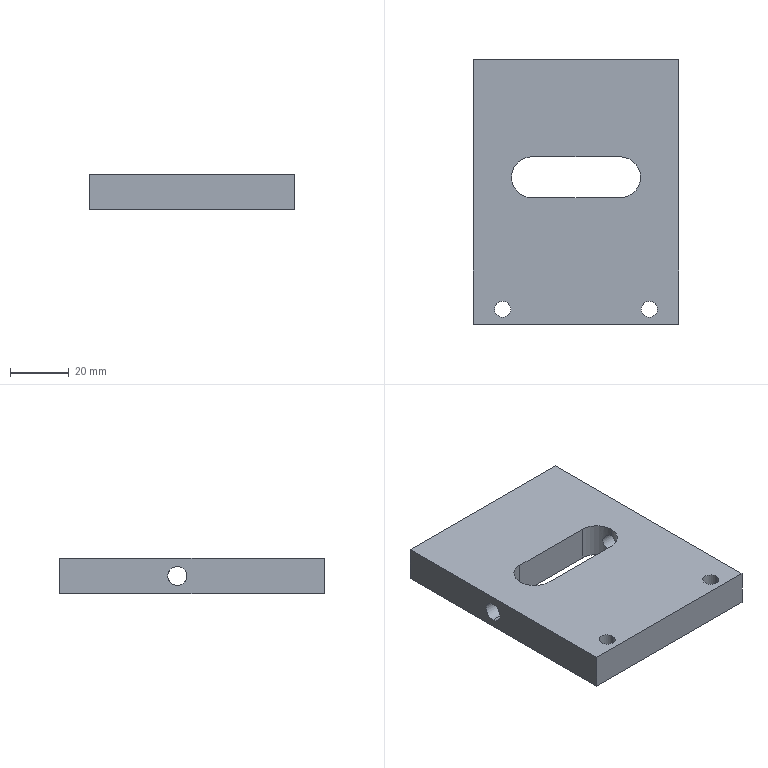Part | SolidWorks | features ICE 2, Cut 1, Extrusion 1, HoleWzd 1 | 1 solid | 27 faces | box 70 x 90 x 12 mm | volume 66580 mm3 | cylinder 15 | plane 8 | cone 4 | commonest cylinder face diameters 5 x4 5.5 x4 6.5 x4 14 x3
STEP:
#1=CARTESIAN_POINT('',(57.25,-85.,0.));
#2=VERTEX_POINT('',#1);
#3=CARTESIAN_POINT('',(62.75,-85.,0.));
#4=VERTEX_POINT('',#3);
#5=CARTESIAN_POINT('',(60.,-85.,0.));
#6=DIRECTION('',(0.,0.,1.));
#7=DIRECTION('',(1.,0.,0.));
#8=AXIS2_PLACEMENT_3D('',#5,#6,#7);
#9=CIRCLE('',#8,2.75);
#10=EDGE_CURVE('',#2,#4,#9,.T.);
#11=ORIENTED_EDGE('',*,*,#10,.F.);
#12=CARTESIAN_POINT('',(57.25,-85.,12.));
#13=VERTEX_POINT('',#12);
#14=CARTESIAN_POINT('',(57.25,-85.,0.));
#15=DIRECTION('',(0.,0.,1.));
#16=VECTOR('',#15,1000.);
#17=LINE('',#14,#16);
#18=EDGE_CURVE('',#2,#13,#17,.T.);
#19=ORIENTED_EDGE('',*,*,#18,.T.);
#20=CARTESIAN_POINT('',(62.75,-85.,12.));
#21=VERTEX_POINT('',#20);
#22=CARTESIAN_POINT('',(60.,-85.,12.));
#23=DIRECTION('',(0.,0.,1.));
#24=DIRECTION('',(1.,0.,0.));
#25=AXIS2_PLACEMENT_3D('',#22,#23,#24);
#26=CIRCLE('',#25,2.75);
#27=EDGE_CURVE('',#13,#21,#26,.T.);
#28=ORIENTED_EDGE('',*,*,#27,.T.);
#29=CARTESIAN_POINT('',(62.75,-85.,0.));
#30=DIRECTION('',(0.,0.,1.));
#31=VECTOR('',#30,1000.);
#32=LINE('',#29,#31);
#33=EDGE_CURVE('',#4,#21,#32,.T.);
#34=ORIENTED_EDGE('',*,*,#33,.F.);
#35=EDGE_LOOP('',(#11,#19,#28,#34));
#36=FACE_OUTER_BOUND('',#35,.T.);
#37=CARTESIAN_POINT('',(60.,-85.,0.));
#38=DIRECTION('',(0.,0.,1.));
#39=DIRECTION('',(1.,0.,0.));
#40=AXIS2_PLACEMENT_3D('',#37,#38,#39);
#41=CYLINDRICAL_SURFACE('',#40,2.75);
#42=ADVANCED_FACE('',(#36),#41,.F.);
#43=CARTESIAN_POINT('',(7.25,-85.,0.));
#44=VERTEX_POINT('',#43);
#45=CARTESIAN_POINT('',(12.75,-85.,0.));
#46=VERTEX_POINT('',#45);
#47=CARTESIAN_POINT('',(10.,-85.,0.));
#48=DIRECTION('',(0.,0.,1.));
#49=DIRECTION('',(1.,0.,0.));
#50=AXIS2_PLACEMENT_3D('',#47,#48,#49);
#51=CIRCLE('',#50,2.75);
#52=EDGE_CURVE('',#44,#46,#51,.T.);
#53=ORIENTED_EDGE('',*,*,#52,.F.);
#54=CARTESIAN_POINT('',(7.25,-85.,12.));
#55=VERTEX_POINT('',#54);
#56=CARTESIAN_POINT('',(7.25,-85.,0.));
#57=DIRECTION('',(0.,0.,1.));
#58=VECTOR('',#57,1000.);
#59=LINE('',#56,#58);
#60=EDGE_CURVE('',#44,#55,#59,.T.);
#61=ORIENTED_EDGE('',*,*,#60,.T.);
#62=CARTESIAN_POINT('',(12.75,-85.,12.));
#63=VERTEX_POINT('',#62);
#64=CARTESIAN_POINT('',(10.,-85.,12.));
#65=DIRECTION('',(0.,0.,1.));
#66=DIRECTION('',(1.,0.,0.));
#67=AXIS2_PLACEMENT_3D('',#64,#65,#66);
#68=CIRCLE('',#67,2.75);
#69=EDGE_CURVE('',#55,#63,#68,.T.);
#70=ORIENTED_EDGE('',*,*,#69,.T.);
#71=CARTESIAN_POINT('',(12.75,-85.,0.));
#72=DIRECTION('',(0.,0.,1.));
#73=VECTOR('',#72,1000.);
#74=LINE('',#71,#73);
#75=EDGE_CURVE('',#46,#63,#74,.T.);
#76=ORIENTED_EDGE('',*,*,#75,.F.);
#77=EDGE_LOOP('',(#53,#61,#70,#76));
#78=FACE_OUTER_BOUND('',#77,.T.);
#79=CARTESIAN_POINT('',(10.,-85.,0.));
#80=DIRECTION('',(0.,0.,1.));
#81=DIRECTION('',(1.,0.,0.));
#82=AXIS2_PLACEMENT_3D('',#79,#80,#81);
#83=CYLINDRICAL_SURFACE('',#82,2.75);
#84=ADVANCED_FACE('',(#78),#83,.F.);
#85=CARTESIAN_POINT('',(62.5,-17.,3.5));
#86=VERTEX_POINT('',#85);
#87=CARTESIAN_POINT('',(62.5,-17.,8.5));
#88=VERTEX_POINT('',#87);
#89=CARTESIAN_POINT('',(62.5,-17.,6.));
#90=DIRECTION('',(0.,1.,0.));
#91=DIRECTION('',(0.,0.,1.));
#92=AXIS2_PLACEMENT_3D('',#89,#90,#91);
#93=CIRCLE('',#92,2.5);
#94=EDGE_CURVE('',#86,#88,#93,.T.);
#95=ORIENTED_EDGE('',*,*,#94,.F.);
#96=CARTESIAN_POINT('',(62.5,0.,3.5));
#97=VERTEX_POINT('',#96);
#98=CARTESIAN_POINT('',(62.5,0.,3.5));
#99=DIRECTION('',(0.,1.,0.));
#100=VECTOR('',#99,1000.);
#101=LINE('',#98,#100);
#102=EDGE_CURVE('',#86,#97,#101,.T.);
#103=ORIENTED_EDGE('',*,*,#102,.T.);
#104=CARTESIAN_POINT('',(62.5,0.,8.5));
#105=VERTEX_POINT('',#104);
#106=CARTESIAN_POINT('',(62.5,0.,6.));
#107=DIRECTION('',(0.,1.,0.));
#108=DIRECTION('',(0.,0.,1.));
#109=AXIS2_PLACEMENT_3D('',#106,#107,#108);
#110=CIRCLE('',#109,2.5);
#111=EDGE_CURVE('',#97,#105,#110,.T.);
#112=ORIENTED_EDGE('',*,*,#111,.T.);
#113=CARTESIAN_POINT('',(62.5,0.,8.5));
#114=DIRECTION('',(0.,1.,0.));
#115=VECTOR('',#114,1000.);
#116=LINE('',#113,#115);
#117=EDGE_CURVE('',#88,#105,#116,.T.);
#118=ORIENTED_EDGE('',*,*,#117,.F.);
#119=EDGE_LOOP('',(#95,#103,#112,#118));
#120=FACE_OUTER_BOUND('',#119,.T.);
#121=CARTESIAN_POINT('',(62.5,0.,6.));
#122=DIRECTION('',(0.,1.,0.));
#123=DIRECTION('',(0.,0.,1.));
#124=AXIS2_PLACEMENT_3D('',#121,#122,#123);
#125=CYLINDRICAL_SURFACE('',#124,2.5);
#126=ADVANCED_FACE('',(#120),#125,.F.);
#127=CARTESIAN_POINT('',(62.5,-18.502,6.));
#128=VERTEX_POINT('',#127);
#129=CARTESIAN_POINT('',(62.5,-17.,8.5));
#130=DIRECTION('',(0.,0.515,0.8572));
#131=VECTOR('',#130,1000.);
#132=LINE('',#129,#131);
#133=EDGE_CURVE('',#128,#88,#132,.T.);
#134=ORIENTED_EDGE('',*,*,#133,.F.);
#135=CARTESIAN_POINT('',(62.5,-17.,3.5));
#136=DIRECTION('',(0.,0.515,-0.8572));
#137=VECTOR('',#136,1000.);
#138=LINE('',#135,#137);
#139=EDGE_CURVE('',#128,#86,#138,.T.);
#140=ORIENTED_EDGE('',*,*,#139,.T.);
#141=ORIENTED_EDGE('',*,*,#94,.T.);
#142=EDGE_LOOP('',(#134,#140,#141));
#143=FACE_OUTER_BOUND('',#142,.T.);
#144=CARTESIAN_POINT('',(62.5,-17.,6.));
#145=DIRECTION('',(0.,1.,0.));
#146=DIRECTION('',(0.,0.,1.));
#147=AXIS2_PLACEMENT_3D('',#144,#145,#146);
#148=CONICAL_SURFACE('',#147,2.5,1.03);
#149=ADVANCED_FACE('',(#143),#148,.F.);
#150=CARTESIAN_POINT('',(7.5,-17.,3.5));
#151=VERTEX_POINT('',#150);
#152=CARTESIAN_POINT('',(7.5,-17.,8.5));
#153=VERTEX_POINT('',#152);
#154=CARTESIAN_POINT('',(7.5,-17.,6.));
#155=DIRECTION('',(0.,1.,0.));
#156=DIRECTION('',(0.,0.,1.));
#157=AXIS2_PLACEMENT_3D('',#154,#155,#156);
#158=CIRCLE('',#157,2.5);
#159=EDGE_CURVE('',#151,#153,#158,.T.);
#160=ORIENTED_EDGE('',*,*,#159,.F.);
#161=CARTESIAN_POINT('',(7.5,0.,3.5));
#162=VERTEX_POINT('',#161);
#163=CARTESIAN_POINT('',(7.5,0.,3.5));
#164=DIRECTION('',(0.,1.,0.));
#165=VECTOR('',#164,1000.);
#166=LINE('',#163,#165);
#167=EDGE_CURVE('',#151,#162,#166,.T.);
#168=ORIENTED_EDGE('',*,*,#167,.T.);
#169=CARTESIAN_POINT('',(7.5,0.,8.5));
#170=VERTEX_POINT('',#169);
#171=CARTESIAN_POINT('',(7.5,0.,6.));
#172=DIRECTION('',(0.,1.,0.));
#173=DIRECTION('',(0.,0.,1.));
#174=AXIS2_PLACEMENT_3D('',#171,#172,#173);
#175=CIRCLE('',#174,2.5);
#176=EDGE_CURVE('',#162,#170,#175,.T.);
#177=ORIENTED_EDGE('',*,*,#176,.T.);
#178=CARTESIAN_POINT('',(7.5,0.,8.5));
#179=DIRECTION('',(0.,1.,0.));
#180=VECTOR('',#179,1000.);
#181=LINE('',#178,#180);
#182=EDGE_CURVE('',#153,#170,#181,.T.);
#183=ORIENTED_EDGE('',*,*,#182,.F.);
#184=EDGE_LOOP('',(#160,#168,#177,#183));
#185=FACE_OUTER_BOUND('',#184,.T.);
#186=CARTESIAN_POINT('',(7.5,0.,6.));
#187=DIRECTION('',(0.,1.,0.));
#188=DIRECTION('',(0.,0.,1.));
#189=AXIS2_PLACEMENT_3D('',#186,#187,#188);
#190=CYLINDRICAL_SURFACE('',#189,2.5);
#191=ADVANCED_FACE('',(#185),#190,.F.);
#192=CARTESIAN_POINT('',(7.5,-18.502,6.));
#193=VERTEX_POINT('',#192);
#194=CARTESIAN_POINT('',(7.5,-17.,8.5));
#195=DIRECTION('',(0.,0.515,0.8572));
#196=VECTOR('',#195,1000.);
#197=LINE('',#194,#196);
#198=EDGE_CURVE('',#193,#153,#197,.T.);
#199=ORIENTED_EDGE('',*,*,#198,.F.);
#200=CARTESIAN_POINT('',(7.5,-17.,3.5));
#201=DIRECTION('',(0.,0.515,-0.8572));
#202=VECTOR('',#201,1000.);
#203=LINE('',#200,#202);
#204=EDGE_CURVE('',#193,#151,#203,.T.);
#205=ORIENTED_EDGE('',*,*,#204,.T.);
#206=ORIENTED_EDGE('',*,*,#159,.T.);
#207=EDGE_LOOP('',(#199,#205,#206));
#208=FACE_OUTER_BOUND('',#207,.T.);
#209=CARTESIAN_POINT('',(7.5,-17.,6.));
#210=DIRECTION('',(0.,1.,0.));
#211=DIRECTION('',(0.,0.,1.));
#212=AXIS2_PLACEMENT_3D('',#209,#210,#211);
#213=CONICAL_SURFACE('',#212,2.5,1.03);
#214=ADVANCED_FACE('',(#208),#213,.F.);
#215=CARTESIAN_POINT('',(0.,-40.,9.25));
#216=VERTEX_POINT('',#215);
#217=CARTESIAN_POINT('',(0.,-40.,2.75));
#218=VERTEX_POINT('',#217);
#219=CARTESIAN_POINT('',(0.,-40.,6.));
#220=DIRECTION('',(1.,0.,0.));
#221=DIRECTION('',(0.,0.,-1.));
#222=AXIS2_PLACEMENT_3D('',#219,#220,#221);
#223=CIRCLE('',#222,3.25);
#224=EDGE_CURVE('',#216,#218,#223,.T.);
#225=ORIENTED_EDGE('',*,*,#224,.F.);
#226=CARTESIAN_POINT('',(13.,-40.,9.25));
#227=VERTEX_POINT('',#226);
#228=CARTESIAN_POINT('',(0.,-40.,9.25));
#229=DIRECTION('',(1.,0.,0.));
#230=VECTOR('',#229,1000.);
#231=LINE('',#228,#230);
#232=EDGE_CURVE('',#216,#227,#231,.T.);
#233=ORIENTED_EDGE('',*,*,#232,.T.);
#234=CARTESIAN_POINT('',(13.,-40.,2.75));
#235=VERTEX_POINT('',#234);
#236=CARTESIAN_POINT('',(13.,-40.,2.75));
#237=CARTESIAN_POINT('',(13.,-40.218,2.75));
#238=CARTESIAN_POINT('',(13.01,-40.432,2.772));
#239=CARTESIAN_POINT('',(13.049,-40.852,2.856));
#240=CARTESIAN_POINT('',(13.078,-41.06,2.92));
#241=CARTESIAN_POINT('',(13.149,-41.453,3.085));
#242=CARTESIAN_POINT('',(13.192,-41.638,3.185));
#243=CARTESIAN_POINT('',(13.286,-41.989,3.421));
#244=CARTESIAN_POINT('',(13.337,-42.153,3.556));
#245=CARTESIAN_POINT('',(13.44,-42.448,3.852));
#246=CARTESIAN_POINT('',(13.492,-42.582,4.015));
#247=CARTESIAN_POINT('',(13.591,-42.817,4.366));
#248=CARTESIAN_POINT('',(13.636,-42.917,4.551));
#249=CARTESIAN_POINT('',(13.713,-43.08,4.94));
#250=CARTESIAN_POINT('',(13.745,-43.144,5.148));
#251=CARTESIAN_POINT('',(13.789,-43.228,5.569));
#252=CARTESIAN_POINT('',(13.8,-43.25,5.782));
#253=CARTESIAN_POINT('',(13.8,-43.25,6.213));
#254=CARTESIAN_POINT('',(13.789,-43.228,6.432));
#255=CARTESIAN_POINT('',(13.745,-43.144,6.852));
#256=CARTESIAN_POINT('',(13.714,-43.081,7.057));
#257=CARTESIAN_POINT('',(13.635,-42.916,7.452));
#258=CARTESIAN_POINT('',(13.59,-42.816,7.637));
#259=CARTESIAN_POINT('',(13.492,-42.581,7.986));
#260=CARTESIAN_POINT('',(13.439,-42.446,8.151));
#261=CARTESIAN_POINT('',(13.336,-42.15,8.446));
#262=CARTESIAN_POINT('',(13.286,-41.988,8.579));
#263=CARTESIAN_POINT('',(13.192,-41.637,8.816));
#264=CARTESIAN_POINT('',(13.149,-41.449,8.917));
#265=CARTESIAN_POINT('',(13.078,-41.059,9.08));
#266=CARTESIAN_POINT('',(13.049,-40.854,9.143));
#267=CARTESIAN_POINT('',(13.01,-40.429,9.229));
#268=CARTESIAN_POINT('',(13.,-40.215,9.25));
#269=CARTESIAN_POINT('',(13.,-40.,9.25));
#270=B_SPLINE_CURVE_WITH_KNOTS('',3,(#236,#237,#238,#239,#240,#241,#242,#243,#244,#245,#246,#247,#248,#249,#250,#251,#252,#253,#254,#255,#256,#257,#258,#259,#260,#261,#262,#263,#264,#265,#266,#267,#268,#269),.UNSPECIFIED.,.F.,.F.,(4,2,2,2,2,2,2,2,2,2,2,2,2,2,2,2,4),(0.,0.0006445,0.001289,0.001933,0.002578,0.003222,0.003867,0.004511,0.005156,0.0058,0.006445,0.007089,0.007733,0.008378,0.009022,0.009667,0.01031),.UNSPECIFIED.);
#271=EDGE_CURVE('',#235,#227,#270,.T.);
#272=ORIENTED_EDGE('',*,*,#271,.F.);
#273=CARTESIAN_POINT('',(0.,-40.,2.75));
#274=DIRECTION('',(1.,0.,0.));
#275=VECTOR('',#274,1000.);
#276=LINE('',#273,#275);
#277=EDGE_CURVE('',#218,#235,#276,.T.);
#278=ORIENTED_EDGE('',*,*,#277,.F.);
#279=EDGE_LOOP('',(#225,#233,#272,#278));
#280=FACE_OUTER_BOUND('',#279,.T.);
#281=CARTESIAN_POINT('',(0.,-40.,6.));
#282=DIRECTION('',(1.,0.,0.));
#283=DIRECTION('',(0.,0.,-1.));
#284=AXIS2_PLACEMENT_3D('',#281,#282,#283);
#285=CYLINDRICAL_SURFACE('',#284,3.25);
#286=ADVANCED_FACE('',(#280),#285,.F.);
#287=CARTESIAN_POINT('',(57.,-40.,9.25));
#288=VERTEX_POINT('',#287);
#289=CARTESIAN_POINT('',(57.,-40.,2.75));
#290=VERTEX_POINT('',#289);
#291=CARTESIAN_POINT('',(57.,-40.,9.25));
#292=CARTESIAN_POINT('',(57.,-40.215,9.25));
#293=CARTESIAN_POINT('',(56.99,-40.433,9.228));
#294=CARTESIAN_POINT('',(56.951,-40.854,9.143));
#295=CARTESIAN_POINT('',(56.922,-41.058,9.08));
#296=CARTESIAN_POINT('',(56.851,-41.453,8.915));
#297=CARTESIAN_POINT('',(56.808,-41.64,8.814));
#298=CARTESIAN_POINT('',(56.714,-41.989,8.579));
#299=CARTESIAN_POINT('',(56.663,-42.153,8.444));
#300=CARTESIAN_POINT('',(56.559,-42.449,8.147));
#301=CARTESIAN_POINT('',(56.508,-42.581,7.986));
#302=CARTESIAN_POINT('',(56.41,-42.815,7.637));
#303=CARTESIAN_POINT('',(56.364,-42.917,7.448));
#304=CARTESIAN_POINT('',(56.287,-43.08,7.058));
#305=CARTESIAN_POINT('',(56.255,-43.143,6.856));
#306=CARTESIAN_POINT('',(56.211,-43.228,6.434));
#307=CARTESIAN_POINT('',(56.2,-43.25,6.217));
#308=CARTESIAN_POINT('',(56.2,-43.25,5.788));
#309=CARTESIAN_POINT('',(56.211,-43.229,5.572));
#310=CARTESIAN_POINT('',(56.255,-43.144,5.148));
#311=CARTESIAN_POINT('',(56.286,-43.081,4.944));
#312=CARTESIAN_POINT('',(56.364,-42.918,4.552));
#313=CARTESIAN_POINT('',(56.41,-42.816,4.364));
#314=CARTESIAN_POINT('',(56.508,-42.582,4.015));
#315=CARTESIAN_POINT('',(56.56,-42.449,3.853));
#316=CARTESIAN_POINT('',(56.663,-42.15,3.554));
#317=CARTESIAN_POINT('',(56.714,-41.989,3.421));
#318=CARTESIAN_POINT('',(56.807,-41.641,3.187));
#319=CARTESIAN_POINT('',(56.851,-41.452,3.085));
#320=CARTESIAN_POINT('',(56.922,-41.059,2.92));
#321=CARTESIAN_POINT('',(56.951,-40.856,2.857));
#322=CARTESIAN_POINT('',(56.99,-40.436,2.772));
#323=CARTESIAN_POINT('',(57.,-40.218,2.75));
#324=CARTESIAN_POINT('',(57.,-40.,2.75));
#325=B_SPLINE_CURVE_WITH_KNOTS('',3,(#291,#292,#293,#294,#295,#296,#297,#298,#299,#300,#301,#302,#303,#304,#305,#306,#307,#308,#309,#310,#311,#312,#313,#314,#315,#316,#317,#318,#319,#320,#321,#322,#323,#324),.UNSPECIFIED.,.F.,.F.,(4,2,2,2,2,2,2,2,2,2,2,2,2,2,2,2,4),(0.01031,0.01095,0.0116,0.01224,0.01289,0.01353,0.01417,0.01482,0.01546,0.0161,0.01675,0.01739,0.01803,0.01868,0.01932,0.01997,0.02061),.UNSPECIFIED.);
#326=EDGE_CURVE('',#288,#290,#325,.T.);
#327=ORIENTED_EDGE('',*,*,#326,.F.);
#328=CARTESIAN_POINT('',(70.,-40.,9.25));
#329=VERTEX_POINT('',#328);
#330=CARTESIAN_POINT('',(0.,-40.,9.25));
#331=DIRECTION('',(1.,0.,0.));
#332=VECTOR('',#331,1000.);
#333=LINE('',#330,#332);
#334=EDGE_CURVE('',#288,#329,#333,.T.);
#335=ORIENTED_EDGE('',*,*,#334,.T.);
#336=CARTESIAN_POINT('',(70.,-40.,2.75));
#337=VERTEX_POINT('',#336);
#338=CARTESIAN_POINT('',(70.,-40.,6.));
#339=DIRECTION('',(1.,0.,0.));
#340=DIRECTION('',(0.,0.,-1.));
#341=AXIS2_PLACEMENT_3D('',#338,#339,#340);
#342=CIRCLE('',#341,3.25);
#343=EDGE_CURVE('',#329,#337,#342,.T.);
#344=ORIENTED_EDGE('',*,*,#343,.T.);
#345=CARTESIAN_POINT('',(0.,-40.,2.75));
#346=DIRECTION('',(1.,0.,0.));
#347=VECTOR('',#346,1000.);
#348=LINE('',#345,#347);
#349=EDGE_CURVE('',#290,#337,#348,.T.);
#350=ORIENTED_EDGE('',*,*,#349,.F.);
#351=EDGE_LOOP('',(#327,#335,#344,#350));
#352=FACE_OUTER_BOUND('',#351,.T.);
#353=CARTESIAN_POINT('',(0.,-40.,6.));
#354=DIRECTION('',(1.,0.,0.));
#355=DIRECTION('',(0.,0.,-1.));
#356=AXIS2_PLACEMENT_3D('',#353,#354,#355);
#357=CYLINDRICAL_SURFACE('',#356,3.25);
#358=ADVANCED_FACE('',(#352),#357,.F.);
#359=CARTESIAN_POINT('',(57.,-40.,0.));
#360=VERTEX_POINT('',#359);
#361=CARTESIAN_POINT('',(50.,-33.,0.));
#362=VERTEX_POINT('',#361);
#363=CARTESIAN_POINT('',(50.,-40.,0.));
#364=DIRECTION('',(0.,0.,1.));
#365=DIRECTION('',(1.,0.,0.));
#366=AXIS2_PLACEMENT_3D('',#363,#364,#365);
#367=CIRCLE('',#366,7.);
#368=EDGE_CURVE('',#360,#362,#367,.T.);
#369=ORIENTED_EDGE('',*,*,#368,.F.);
#370=CARTESIAN_POINT('',(57.,-40.,0.));
#371=DIRECTION('',(0.,0.,1.));
#372=VECTOR('',#371,1000.);
#373=LINE('',#370,#372);
#374=EDGE_CURVE('',#360,#290,#373,.T.);
#375=ORIENTED_EDGE('',*,*,#374,.T.);
#376=CARTESIAN_POINT('',(57.,-40.,2.75));
#377=CARTESIAN_POINT('',(57.,-39.782,2.75));
#378=CARTESIAN_POINT('',(56.99,-39.568,2.772));
#379=CARTESIAN_POINT('',(56.951,-39.148,2.856));
#380=CARTESIAN_POINT('',(56.922,-38.94,2.92));
#381=CARTESIAN_POINT('',(56.851,-38.547,3.085));
#382=CARTESIAN_POINT('',(56.808,-38.362,3.185));
#383=CARTESIAN_POINT('',(56.714,-38.011,3.421));
#384=CARTESIAN_POINT('',(56.663,-37.847,3.556));
#385=CARTESIAN_POINT('',(56.56,-37.552,3.852));
#386=CARTESIAN_POINT('',(56.508,-37.418,4.015));
#387=CARTESIAN_POINT('',(56.409,-37.183,4.366));
#388=CARTESIAN_POINT('',(56.364,-37.083,4.551));
#389=CARTESIAN_POINT('',(56.287,-36.92,4.94));
#390=CARTESIAN_POINT('',(56.255,-36.856,5.148));
#391=CARTESIAN_POINT('',(56.211,-36.772,5.569));
#392=CARTESIAN_POINT('',(56.2,-36.75,5.782));
#393=CARTESIAN_POINT('',(56.2,-36.75,6.213));
#394=CARTESIAN_POINT('',(56.211,-36.772,6.432));
#395=CARTESIAN_POINT('',(56.255,-36.856,6.852));
#396=CARTESIAN_POINT('',(56.286,-36.919,7.057));
#397=CARTESIAN_POINT('',(56.365,-37.084,7.452));
#398=CARTESIAN_POINT('',(56.41,-37.184,7.637));
#399=CARTESIAN_POINT('',(56.508,-37.419,7.986));
#400=CARTESIAN_POINT('',(56.561,-37.554,8.151));
#401=CARTESIAN_POINT('',(56.664,-37.85,8.446));
#402=CARTESIAN_POINT('',(56.714,-38.012,8.579));
#403=CARTESIAN_POINT('',(56.808,-38.363,8.816));
#404=CARTESIAN_POINT('',(56.851,-38.551,8.917));
#405=CARTESIAN_POINT('',(56.922,-38.941,9.08));
#406=CARTESIAN_POINT('',(56.951,-39.146,9.143));
#407=CARTESIAN_POINT('',(56.99,-39.571,9.229));
#408=CARTESIAN_POINT('',(57.,-39.785,9.25));
#409=CARTESIAN_POINT('',(57.,-40.,9.25));
#410=B_SPLINE_CURVE_WITH_KNOTS('',3,(#376,#377,#378,#379,#380,#381,#382,#383,#384,#385,#386,#387,#388,#389,#390,#391,#392,#393,#394,#395,#396,#397,#398,#399,#400,#401,#402,#403,#404,#405,#406,#407,#408,#409),.UNSPECIFIED.,.F.,.F.,(4,2,2,2,2,2,2,2,2,2,2,2,2,2,2,2,4),(0.,0.0006445,0.001289,0.001933,0.002578,0.003222,0.003867,0.004511,0.005156,0.0058,0.006445,0.007089,0.007733,0.008378,0.009022,0.009667,0.01031),.UNSPECIFIED.);
#411=EDGE_CURVE('',#290,#288,#410,.T.);
#412=ORIENTED_EDGE('',*,*,#411,.T.);
#413=CARTESIAN_POINT('',(57.,-40.,12.));
#414=VERTEX_POINT('',#413);
#415=CARTESIAN_POINT('',(57.,-40.,0.));
#416=DIRECTION('',(0.,0.,1.));
#417=VECTOR('',#416,1000.);
#418=LINE('',#415,#417);
#419=EDGE_CURVE('',#288,#414,#418,.T.);
#420=ORIENTED_EDGE('',*,*,#419,.T.);
#421=CARTESIAN_POINT('',(50.,-33.,12.));
#422=VERTEX_POINT('',#421);
#423=CARTESIAN_POINT('',(50.,-40.,12.));
#424=DIRECTION('',(0.,0.,1.));
#425=DIRECTION('',(1.,0.,0.));
#426=AXIS2_PLACEMENT_3D('',#423,#424,#425);
#427=CIRCLE('',#426,7.);
#428=EDGE_CURVE('',#414,#422,#427,.T.);
#429=ORIENTED_EDGE('',*,*,#428,.T.);
#430=CARTESIAN_POINT('',(50.,-33.,0.));
#431=DIRECTION('',(0.,0.,1.));
#432=VECTOR('',#431,1000.);
#433=LINE('',#430,#432);
#434=EDGE_CURVE('',#362,#422,#433,.T.);
#435=ORIENTED_EDGE('',*,*,#434,.F.);
#436=EDGE_LOOP('',(#369,#375,#412,#420,#429,#435));
#437=FACE_OUTER_BOUND('',#436,.T.);
#438=CARTESIAN_POINT('',(50.,-40.,0.));
#439=DIRECTION('',(0.,0.,1.));
#440=DIRECTION('',(1.,0.,0.));
#441=AXIS2_PLACEMENT_3D('',#438,#439,#440);
#442=CYLINDRICAL_SURFACE('',#441,7.);
#443=ADVANCED_FACE('',(#437),#442,.F.);
#444=CARTESIAN_POINT('',(0.,-40.,6.));
#445=DIRECTION('',(1.,0.,0.));
#446=DIRECTION('',(0.,0.,-1.));
#447=AXIS2_PLACEMENT_3D('',#444,#445,#446);
#448=CIRCLE('',#447,3.25);
#449=EDGE_CURVE('',#218,#216,#448,.T.);
#450=ORIENTED_EDGE('',*,*,#449,.T.);
#451=ORIENTED_EDGE('',*,*,#224,.T.);
#452=EDGE_LOOP('',(#450,#451));
#453=FACE_BOUND('',#452,.T.);
#454=CARTESIAN_POINT('',(0.,0.,0.));
#455=VERTEX_POINT('',#454);
#456=CARTESIAN_POINT('',(0.,-90.,0.));
#457=VERTEX_POINT('',#456);
#458=CARTESIAN_POINT('',(0.,0.,0.));
#459=DIRECTION('',(0.,-1.,0.));
#460=VECTOR('',#459,1000.);
#461=LINE('',#458,#460);
#462=EDGE_CURVE('',#455,#457,#461,.T.);
#463=ORIENTED_EDGE('',*,*,#462,.T.);
#464=CARTESIAN_POINT('',(0.,-90.,12.));
#465=VERTEX_POINT('',#464);
#466=CARTESIAN_POINT('',(0.,-90.,12.));
#467=DIRECTION('',(0.,0.,-1.));
#468=VECTOR('',#467,1000.);
#469=LINE('',#466,#468);
#470=EDGE_CURVE('',#465,#457,#469,.T.);
#471=ORIENTED_EDGE('',*,*,#470,.F.);
#472=CARTESIAN_POINT('',(0.,0.,12.));
#473=VERTEX_POINT('',#472);
#474=CARTESIAN_POINT('',(0.,0.,12.));
#475=DIRECTION('',(0.,-1.,0.));
#476=VECTOR('',#475,1000.);
#477=LINE('',#474,#476);
#478=EDGE_CURVE('',#473,#465,#477,.T.);
#479=ORIENTED_EDGE('',*,*,#478,.F.);
#480=CARTESIAN_POINT('',(0.,0.,12.));
#481=DIRECTION('',(0.,0.,-1.));
#482=VECTOR('',#481,1000.);
#483=LINE('',#480,#482);
#484=EDGE_CURVE('',#473,#455,#483,.T.);
#485=ORIENTED_EDGE('',*,*,#484,.T.);
#486=EDGE_LOOP('',(#463,#471,#479,#485));
#487=FACE_OUTER_BOUND('',#486,.T.);
#488=CARTESIAN_POINT('',(0.,0.,12.));
#489=DIRECTION('',(1.,0.,0.));
#490=DIRECTION('',(0.,1.,0.));
#491=AXIS2_PLACEMENT_3D('',#488,#489,#490);
#492=PLANE('',#491);
#493=ADVANCED_FACE('',(#453,#487),#492,.F.);
#494=CARTESIAN_POINT('',(70.,-90.,0.));
#495=VERTEX_POINT('',#494);
#496=CARTESIAN_POINT('',(0.,-90.,0.));
#497=DIRECTION('',(1.,0.,0.));
#498=VECTOR('',#497,1000.);
#499=LINE('',#496,#498);
#500=EDGE_CURVE('',#457,#495,#499,.T.);
#501=ORIENTED_EDGE('',*,*,#500,.T.);
#502=CARTESIAN_POINT('',(70.,-90.,12.));
#503=VERTEX_POINT('',#502);
#504=CARTESIAN_POINT('',(70.,-90.,12.));
#505=DIRECTION('',(0.,0.,-1.));
#506=VECTOR('',#505,1000.);
#507=LINE('',#504,#506);
#508=EDGE_CURVE('',#503,#495,#507,.T.);
#509=ORIENTED_EDGE('',*,*,#508,.F.);
#510=CARTESIAN_POINT('',(0.,-90.,12.));
#511=DIRECTION('',(1.,0.,0.));
#512=VECTOR('',#511,1000.);
#513=LINE('',#510,#512);
#514=EDGE_CURVE('',#465,#503,#513,.T.);
#515=ORIENTED_EDGE('',*,*,#514,.F.);
#516=ORIENTED_EDGE('',*,*,#470,.T.);
#517=EDGE_LOOP('',(#501,#509,#515,#516));
#518=FACE_OUTER_BOUND('',#517,.T.);
#519=CARTESIAN_POINT('',(0.,-90.,12.));
#520=DIRECTION('',(0.,1.,0.));
#521=DIRECTION('',(0.,0.,1.));
#522=AXIS2_PLACEMENT_3D('',#519,#520,#521);
#523=PLANE('',#522);
#524=ADVANCED_FACE('',(#518),#523,.F.);
#525=CARTESIAN_POINT('',(70.,-40.,6.));
#526=DIRECTION('',(1.,0.,0.));
#527=DIRECTION('',(0.,0.,-1.));
#528=AXIS2_PLACEMENT_3D('',#525,#526,#527);
#529=CIRCLE('',#528,3.25);
#530=EDGE_CURVE('',#337,#329,#529,.T.);
#531=ORIENTED_EDGE('',*,*,#530,.F.);
#532=ORIENTED_EDGE('',*,*,#343,.F.);
#533=EDGE_LOOP('',(#531,#532));
#534=FACE_BOUND('',#533,.T.);
#535=CARTESIAN_POINT('',(70.,0.,0.));
#536=VERTEX_POINT('',#535);
#537=CARTESIAN_POINT('',(70.,0.,0.));
#538=DIRECTION('',(0.,1.,0.));
#539=VECTOR('',#538,1000.);
#540=LINE('',#537,#539);
#541=EDGE_CURVE('',#495,#536,#540,.T.);
#542=ORIENTED_EDGE('',*,*,#541,.T.);
#543=CARTESIAN_POINT('',(70.,0.,12.));
#544=VERTEX_POINT('',#543);
#545=CARTESIAN_POINT('',(70.,0.,12.));
#546=DIRECTION('',(0.,0.,-1.));
#547=VECTOR('',#546,1000.);
#548=LINE('',#545,#547);
#549=EDGE_CURVE('',#544,#536,#548,.T.);
#550=ORIENTED_EDGE('',*,*,#549,.F.);
#551=CARTESIAN_POINT('',(70.,0.,12.));
#552=DIRECTION('',(0.,1.,0.));
#553=VECTOR('',#552,1000.);
#554=LINE('',#551,#553);
#555=EDGE_CURVE('',#503,#544,#554,.T.);
#556=ORIENTED_EDGE('',*,*,#555,.F.);
#557=ORIENTED_EDGE('',*,*,#508,.T.);
#558=EDGE_LOOP('',(#542,#550,#556,#557));
#559=FACE_OUTER_BOUND('',#558,.T.);
#560=CARTESIAN_POINT('',(70.,0.,12.));
#561=DIRECTION('',(-1.,0.,0.));
#562=DIRECTION('',(0.,0.,1.));
#563=AXIS2_PLACEMENT_3D('',#560,#561,#562);
#564=PLANE('',#563);
#565=ADVANCED_FACE('',(#534,#559),#564,.F.);
#566=CARTESIAN_POINT('',(62.5,0.,6.));
#567=DIRECTION('',(0.,1.,0.));
#568=DIRECTION('',(0.,0.,1.));
#569=AXIS2_PLACEMENT_3D('',#566,#567,#568);
#570=CIRCLE('',#569,2.5);
#571=EDGE_CURVE('',#105,#97,#570,.T.);
#572=ORIENTED_EDGE('',*,*,#571,.F.);
#573=ORIENTED_EDGE('',*,*,#111,.F.);
#574=EDGE_LOOP('',(#572,#573));
#575=FACE_BOUND('',#574,.T.);
#576=CARTESIAN_POINT('',(7.5,0.,6.));
#577=DIRECTION('',(0.,1.,0.));
#578=DIRECTION('',(0.,0.,1.));
#579=AXIS2_PLACEMENT_3D('',#576,#577,#578);
#580=CIRCLE('',#579,2.5);
#581=EDGE_CURVE('',#170,#162,#580,.T.);
#582=ORIENTED_EDGE('',*,*,#581,.F.);
#583=ORIENTED_EDGE('',*,*,#176,.F.);
#584=EDGE_LOOP('',(#582,#583));
#585=FACE_BOUND('',#584,.T.);
#586=CARTESIAN_POINT('',(0.,0.,0.));
#587=DIRECTION('',(-1.,0.,0.));
#588=VECTOR('',#587,1000.);
#589=LINE('',#586,#588);
#590=EDGE_CURVE('',#536,#455,#589,.T.);
#591=ORIENTED_EDGE('',*,*,#590,.T.);
#592=ORIENTED_EDGE('',*,*,#484,.F.);
#593=CARTESIAN_POINT('',(0.,0.,12.));
#594=DIRECTION('',(-1.,0.,0.));
#595=VECTOR('',#594,1000.);
#596=LINE('',#593,#595);
#597=EDGE_CURVE('',#544,#473,#596,.T.);
#598=ORIENTED_EDGE('',*,*,#597,.F.);
#599=ORIENTED_EDGE('',*,*,#549,.T.);
#600=EDGE_LOOP('',(#591,#592,#598,#599));
#601=FACE_OUTER_BOUND('',#600,.T.);
#602=CARTESIAN_POINT('',(0.,0.,12.));
#603=DIRECTION('',(0.,-1.,0.));
#604=DIRECTION('',(0.,0.,-1.));
#605=AXIS2_PLACEMENT_3D('',#602,#603,#604);
#606=PLANE('',#605);
#607=ADVANCED_FACE('',(#575,#585,#601),#606,.F.);
#608=CARTESIAN_POINT('',(60.,-85.,12.));
#609=DIRECTION('',(0.,0.,1.));
#610=DIRECTION('',(1.,0.,0.));
#611=AXIS2_PLACEMENT_3D('',#608,#609,#610);
#612=CIRCLE('',#611,2.75);
#613=EDGE_CURVE('',#21,#13,#612,.T.);
#614=ORIENTED_EDGE('',*,*,#613,.F.);
#615=ORIENTED_EDGE('',*,*,#27,.F.);
#616=EDGE_LOOP('',(#614,#615));
#617=FACE_BOUND('',#616,.T.);
#618=CARTESIAN_POINT('',(10.,-85.,12.));
#619=DIRECTION('',(0.,0.,1.));
#620=DIRECTION('',(1.,0.,0.));
#621=AXIS2_PLACEMENT_3D('',#618,#619,#620);
#622=CIRCLE('',#621,2.75);
#623=EDGE_CURVE('',#63,#55,#622,.T.);
#624=ORIENTED_EDGE('',*,*,#623,.F.);
#625=ORIENTED_EDGE('',*,*,#69,.F.);
#626=EDGE_LOOP('',(#624,#625));
#627=FACE_BOUND('',#626,.T.);
#628=CARTESIAN_POINT('',(20.,-33.,12.));
#629=VERTEX_POINT('',#628);
#630=CARTESIAN_POINT('',(20.,-47.,12.));
#631=VERTEX_POINT('',#630);
#632=CARTESIAN_POINT('',(20.,-40.,12.));
#633=DIRECTION('',(0.,0.,1.));
#634=DIRECTION('',(1.,0.,0.));
#635=AXIS2_PLACEMENT_3D('',#632,#633,#634);
#636=CIRCLE('',#635,7.);
#637=EDGE_CURVE('',#629,#631,#636,.T.);
#638=ORIENTED_EDGE('',*,*,#637,.F.);
#639=CARTESIAN_POINT('',(20.,-33.,12.));
#640=DIRECTION('',(-1.,0.,0.));
#641=VECTOR('',#640,1000.);
#642=LINE('',#639,#641);
#643=EDGE_CURVE('',#422,#629,#642,.T.);
#644=ORIENTED_EDGE('',*,*,#643,.F.);
#645=ORIENTED_EDGE('',*,*,#428,.F.);
#646=CARTESIAN_POINT('',(50.,-47.,12.));
#647=VERTEX_POINT('',#646);
#648=CARTESIAN_POINT('',(50.,-40.,12.));
#649=DIRECTION('',(0.,0.,1.));
#650=DIRECTION('',(1.,0.,0.));
#651=AXIS2_PLACEMENT_3D('',#648,#649,#650);
#652=CIRCLE('',#651,7.);
#653=EDGE_CURVE('',#647,#414,#652,.T.);
#654=ORIENTED_EDGE('',*,*,#653,.F.);
#655=CARTESIAN_POINT('',(20.,-47.,12.));
#656=DIRECTION('',(1.,0.,0.));
#657=VECTOR('',#656,1000.);
#658=LINE('',#655,#657);
#659=EDGE_CURVE('',#631,#647,#658,.T.);
#660=ORIENTED_EDGE('',*,*,#659,.F.);
#661=EDGE_LOOP('',(#638,#644,#645,#654,#660));
#662=FACE_BOUND('',#661,.T.);
#663=ORIENTED_EDGE('',*,*,#478,.T.);
#664=ORIENTED_EDGE('',*,*,#514,.T.);
#665=ORIENTED_EDGE('',*,*,#555,.T.);
#666=ORIENTED_EDGE('',*,*,#597,.T.);
#667=EDGE_LOOP('',(#663,#664,#665,#666));
#668=FACE_OUTER_BOUND('',#667,.T.);
#669=CARTESIAN_POINT('',(0.,0.,12.));
#670=DIRECTION('',(0.,0.,1.));
#671=DIRECTION('',(1.,0.,0.));
#672=AXIS2_PLACEMENT_3D('',#669,#670,#671);
#673=PLANE('',#672);
#674=ADVANCED_FACE('',(#617,#627,#662,#668),#673,.T.);
#675=CARTESIAN_POINT('',(60.,-85.,0.));
#676=DIRECTION('',(0.,0.,1.));
#677=DIRECTION('',(1.,0.,0.));
#678=AXIS2_PLACEMENT_3D('',#675,#676,#677);
#679=CIRCLE('',#678,2.75);
#680=EDGE_CURVE('',#4,#2,#679,.T.);
#681=ORIENTED_EDGE('',*,*,#680,.T.);
#682=ORIENTED_EDGE('',*,*,#10,.T.);
#683=EDGE_LOOP('',(#681,#682));
#684=FACE_BOUND('',#683,.T.);
#685=CARTESIAN_POINT('',(10.,-85.,0.));
#686=DIRECTION('',(0.,0.,1.));
#687=DIRECTION('',(1.,0.,0.));
#688=AXIS2_PLACEMENT_3D('',#685,#686,#687);
#689=CIRCLE('',#688,2.75);
#690=EDGE_CURVE('',#46,#44,#689,.T.);
#691=ORIENTED_EDGE('',*,*,#690,.T.);
#692=ORIENTED_EDGE('',*,*,#52,.T.);
#693=EDGE_LOOP('',(#691,#692));
#694=FACE_BOUND('',#693,.T.);
#695=CARTESIAN_POINT('',(20.,-33.,0.));
#696=VERTEX_POINT('',#695);
#697=CARTESIAN_POINT('',(20.,-33.,0.));
#698=DIRECTION('',(-1.,0.,0.));
#699=VECTOR('',#698,1000.);
#700=LINE('',#697,#699);
#701=EDGE_CURVE('',#362,#696,#700,.T.);
#702=ORIENTED_EDGE('',*,*,#701,.T.);
#703=CARTESIAN_POINT('',(20.,-47.,0.));
#704=VERTEX_POINT('',#703);
#705=CARTESIAN_POINT('',(20.,-40.,0.));
#706=DIRECTION('',(0.,0.,1.));
#707=DIRECTION('',(1.,0.,0.));
#708=AXIS2_PLACEMENT_3D('',#705,#706,#707);
#709=CIRCLE('',#708,7.);
#710=EDGE_CURVE('',#696,#704,#709,.T.);
#711=ORIENTED_EDGE('',*,*,#710,.T.);
#712=CARTESIAN_POINT('',(50.,-47.,0.));
#713=VERTEX_POINT('',#712);
#714=CARTESIAN_POINT('',(20.,-47.,0.));
#715=DIRECTION('',(1.,0.,0.));
#716=VECTOR('',#715,1000.);
#717=LINE('',#714,#716);
#718=EDGE_CURVE('',#704,#713,#717,.T.);
#719=ORIENTED_EDGE('',*,*,#718,.T.);
#720=CARTESIAN_POINT('',(50.,-40.,0.));
#721=DIRECTION('',(0.,0.,1.));
#722=DIRECTION('',(1.,0.,0.));
#723=AXIS2_PLACEMENT_3D('',#720,#721,#722);
#724=CIRCLE('',#723,7.);
#725=EDGE_CURVE('',#713,#360,#724,.T.);
#726=ORIENTED_EDGE('',*,*,#725,.T.);
#727=ORIENTED_EDGE('',*,*,#368,.T.);
#728=EDGE_LOOP('',(#702,#711,#719,#726,#727));
#729=FACE_BOUND('',#728,.T.);
#730=ORIENTED_EDGE('',*,*,#462,.F.);
#731=ORIENTED_EDGE('',*,*,#590,.F.);
#732=ORIENTED_EDGE('',*,*,#541,.F.);
#733=ORIENTED_EDGE('',*,*,#500,.F.);
#734=EDGE_LOOP('',(#730,#731,#732,#733));
#735=FACE_OUTER_BOUND('',#734,.T.);
#736=CARTESIAN_POINT('',(0.,0.,0.));
#737=DIRECTION('',(0.,0.,1.));
#738=DIRECTION('',(1.,0.,0.));
#739=AXIS2_PLACEMENT_3D('',#736,#737,#738);
#740=PLANE('',#739);
#741=ADVANCED_FACE('',(#684,#694,#729,#735),#740,.F.);
#742=ORIENTED_EDGE('',*,*,#271,.T.);
#743=CARTESIAN_POINT('',(13.,-40.,9.25));
#744=CARTESIAN_POINT('',(13.,-39.785,9.25));
#745=CARTESIAN_POINT('',(13.01,-39.567,9.228));
#746=CARTESIAN_POINT('',(13.049,-39.146,9.143));
#747=CARTESIAN_POINT('',(13.078,-38.942,9.08));
#748=CARTESIAN_POINT('',(13.149,-38.547,8.915));
#749=CARTESIAN_POINT('',(13.192,-38.36,8.814));
#750=CARTESIAN_POINT('',(13.286,-38.011,8.579));
#751=CARTESIAN_POINT('',(13.337,-37.847,8.444));
#752=CARTESIAN_POINT('',(13.441,-37.551,8.147));
#753=CARTESIAN_POINT('',(13.492,-37.419,7.986));
#754=CARTESIAN_POINT('',(13.59,-37.185,7.637));
#755=CARTESIAN_POINT('',(13.636,-37.083,7.448));
#756=CARTESIAN_POINT('',(13.713,-36.92,7.058));
#757=CARTESIAN_POINT('',(13.745,-36.857,6.856));
#758=CARTESIAN_POINT('',(13.789,-36.772,6.434));
#759=CARTESIAN_POINT('',(13.8,-36.75,6.217));
#760=CARTESIAN_POINT('',(13.8,-36.75,5.788));
#761=CARTESIAN_POINT('',(13.789,-36.771,5.572));
#762=CARTESIAN_POINT('',(13.745,-36.856,5.148));
#763=CARTESIAN_POINT('',(13.714,-36.919,4.944));
#764=CARTESIAN_POINT('',(13.636,-37.082,4.552));
#765=CARTESIAN_POINT('',(13.59,-37.184,4.364));
#766=CARTESIAN_POINT('',(13.492,-37.418,4.015));
#767=CARTESIAN_POINT('',(13.44,-37.551,3.853));
#768=CARTESIAN_POINT('',(13.337,-37.85,3.554));
#769=CARTESIAN_POINT('',(13.286,-38.011,3.421));
#770=CARTESIAN_POINT('',(13.193,-38.359,3.187));
#771=CARTESIAN_POINT('',(13.149,-38.548,3.085));
#772=CARTESIAN_POINT('',(13.078,-38.941,2.92));
#773=CARTESIAN_POINT('',(13.049,-39.144,2.857));
#774=CARTESIAN_POINT('',(13.01,-39.564,2.772));
#775=CARTESIAN_POINT('',(13.,-39.782,2.75));
#776=CARTESIAN_POINT('',(13.,-40.,2.75));
#777=B_SPLINE_CURVE_WITH_KNOTS('',3,(#743,#744,#745,#746,#747,#748,#749,#750,#751,#752,#753,#754,#755,#756,#757,#758,#759,#760,#761,#762,#763,#764,#765,#766,#767,#768,#769,#770,#771,#772,#773,#774,#775,#776),.UNSPECIFIED.,.F.,.F.,(4,2,2,2,2,2,2,2,2,2,2,2,2,2,2,2,4),(0.01031,0.01095,0.0116,0.01224,0.01289,0.01353,0.01417,0.01482,0.01546,0.0161,0.01675,0.01739,0.01803,0.01868,0.01932,0.01997,0.02061),.UNSPECIFIED.);
#778=EDGE_CURVE('',#227,#235,#777,.T.);
#779=ORIENTED_EDGE('',*,*,#778,.T.);
#780=EDGE_LOOP('',(#742,#779));
#781=FACE_BOUND('',#780,.T.);
#782=ORIENTED_EDGE('',*,*,#637,.T.);
#783=CARTESIAN_POINT('',(20.,-47.,0.));
#784=DIRECTION('',(0.,0.,1.));
#785=VECTOR('',#784,1000.);
#786=LINE('',#783,#785);
#787=EDGE_CURVE('',#704,#631,#786,.T.);
#788=ORIENTED_EDGE('',*,*,#787,.F.);
#789=ORIENTED_EDGE('',*,*,#710,.F.);
#790=CARTESIAN_POINT('',(20.,-33.,0.));
#791=DIRECTION('',(0.,0.,1.));
#792=VECTOR('',#791,1000.);
#793=LINE('',#790,#792);
#794=EDGE_CURVE('',#696,#629,#793,.T.);
#795=ORIENTED_EDGE('',*,*,#794,.T.);
#796=EDGE_LOOP('',(#782,#788,#789,#795));
#797=FACE_OUTER_BOUND('',#796,.T.);
#798=CARTESIAN_POINT('',(20.,-40.,0.));
#799=DIRECTION('',(0.,0.,1.));
#800=DIRECTION('',(1.,0.,0.));
#801=AXIS2_PLACEMENT_3D('',#798,#799,#800);
#802=CYLINDRICAL_SURFACE('',#801,7.);
#803=ADVANCED_FACE('',(#781,#797),#802,.F.);
#804=ORIENTED_EDGE('',*,*,#643,.T.);
#805=ORIENTED_EDGE('',*,*,#794,.F.);
#806=ORIENTED_EDGE('',*,*,#701,.F.);
#807=ORIENTED_EDGE('',*,*,#434,.T.);
#808=EDGE_LOOP('',(#804,#805,#806,#807));
#809=FACE_OUTER_BOUND('',#808,.T.);
#810=CARTESIAN_POINT('',(20.,-33.,0.));
#811=DIRECTION('',(0.,1.,0.));
#812=DIRECTION('',(0.,0.,1.));
#813=AXIS2_PLACEMENT_3D('',#810,#811,#812);
#814=PLANE('',#813);
#815=ADVANCED_FACE('',(#809),#814,.F.);
#816=ORIENTED_EDGE('',*,*,#374,.F.);
#817=ORIENTED_EDGE('',*,*,#725,.F.);
#818=CARTESIAN_POINT('',(50.,-47.,0.));
#819=DIRECTION('',(0.,0.,1.));
#820=VECTOR('',#819,1000.);
#821=LINE('',#818,#820);
#822=EDGE_CURVE('',#713,#647,#821,.T.);
#823=ORIENTED_EDGE('',*,*,#822,.T.);
#824=ORIENTED_EDGE('',*,*,#653,.T.);
#825=ORIENTED_EDGE('',*,*,#419,.F.);
#826=ORIENTED_EDGE('',*,*,#326,.T.);
#827=EDGE_LOOP('',(#816,#817,#823,#824,#825,#826));
#828=FACE_OUTER_BOUND('',#827,.T.);
#829=CARTESIAN_POINT('',(50.,-40.,0.));
#830=DIRECTION('',(0.,0.,1.));
#831=DIRECTION('',(1.,0.,0.));
#832=AXIS2_PLACEMENT_3D('',#829,#830,#831);
#833=CYLINDRICAL_SURFACE('',#832,7.);
#834=ADVANCED_FACE('',(#828),#833,.F.);
#835=ORIENTED_EDGE('',*,*,#659,.T.);
#836=ORIENTED_EDGE('',*,*,#822,.F.);
#837=ORIENTED_EDGE('',*,*,#718,.F.);
#838=ORIENTED_EDGE('',*,*,#787,.T.);
#839=EDGE_LOOP('',(#835,#836,#837,#838));
#840=FACE_OUTER_BOUND('',#839,.T.);
#841=CARTESIAN_POINT('',(20.,-47.,0.));
#842=DIRECTION('',(0.,-1.,0.));
#843=DIRECTION('',(1.,0.,0.));
#844=AXIS2_PLACEMENT_3D('',#841,#842,#843);
#845=PLANE('',#844);
#846=ADVANCED_FACE('',(#840),#845,.F.);
#847=ORIENTED_EDGE('',*,*,#334,.F.);
#848=ORIENTED_EDGE('',*,*,#411,.F.);
#849=ORIENTED_EDGE('',*,*,#349,.T.);
#850=ORIENTED_EDGE('',*,*,#530,.T.);
#851=EDGE_LOOP('',(#847,#848,#849,#850));
#852=FACE_OUTER_BOUND('',#851,.T.);
#853=CARTESIAN_POINT('',(0.,-40.,6.));
#854=DIRECTION('',(1.,0.,0.));
#855=DIRECTION('',(0.,0.,-1.));
#856=AXIS2_PLACEMENT_3D('',#853,#854,#855);
#857=CYLINDRICAL_SURFACE('',#856,3.25);
#858=ADVANCED_FACE('',(#852),#857,.F.);
#859=ORIENTED_EDGE('',*,*,#232,.F.);
#860=ORIENTED_EDGE('',*,*,#449,.F.);
#861=ORIENTED_EDGE('',*,*,#277,.T.);
#862=ORIENTED_EDGE('',*,*,#778,.F.);
#863=EDGE_LOOP('',(#859,#860,#861,#862));
#864=FACE_OUTER_BOUND('',#863,.T.);
#865=CARTESIAN_POINT('',(0.,-40.,6.));
#866=DIRECTION('',(1.,0.,0.));
#867=DIRECTION('',(0.,0.,-1.));
#868=AXIS2_PLACEMENT_3D('',#865,#866,#867);
#869=CYLINDRICAL_SURFACE('',#868,3.25);
#870=ADVANCED_FACE('',(#864),#869,.F.);
#871=ORIENTED_EDGE('',*,*,#204,.F.);
#872=ORIENTED_EDGE('',*,*,#198,.T.);
#873=CARTESIAN_POINT('',(7.5,-17.,6.));
#874=DIRECTION('',(0.,1.,0.));
#875=DIRECTION('',(0.,0.,1.));
#876=AXIS2_PLACEMENT_3D('',#873,#874,#875);
#877=CIRCLE('',#876,2.5);
#878=EDGE_CURVE('',#153,#151,#877,.T.);
#879=ORIENTED_EDGE('',*,*,#878,.T.);
#880=EDGE_LOOP('',(#871,#872,#879));
#881=FACE_OUTER_BOUND('',#880,.T.);
#882=CARTESIAN_POINT('',(7.5,-17.,6.));
#883=DIRECTION('',(0.,1.,0.));
#884=DIRECTION('',(0.,0.,1.));
#885=AXIS2_PLACEMENT_3D('',#882,#883,#884);
#886=CONICAL_SURFACE('',#885,2.5,1.03);
#887=ADVANCED_FACE('',(#881),#886,.F.);
#888=ORIENTED_EDGE('',*,*,#167,.F.);
#889=ORIENTED_EDGE('',*,*,#878,.F.);
#890=ORIENTED_EDGE('',*,*,#182,.T.);
#891=ORIENTED_EDGE('',*,*,#581,.T.);
#892=EDGE_LOOP('',(#888,#889,#890,#891));
#893=FACE_OUTER_BOUND('',#892,.T.);
#894=CARTESIAN_POINT('',(7.5,0.,6.));
#895=DIRECTION('',(0.,1.,0.));
#896=DIRECTION('',(0.,0.,1.));
#897=AXIS2_PLACEMENT_3D('',#894,#895,#896);
#898=CYLINDRICAL_SURFACE('',#897,2.5);
#899=ADVANCED_FACE('',(#893),#898,.F.);
#900=ORIENTED_EDGE('',*,*,#139,.F.);
#901=ORIENTED_EDGE('',*,*,#133,.T.);
#902=CARTESIAN_POINT('',(62.5,-17.,6.));
#903=DIRECTION('',(0.,1.,0.));
#904=DIRECTION('',(0.,0.,1.));
#905=AXIS2_PLACEMENT_3D('',#902,#903,#904);
#906=CIRCLE('',#905,2.5);
#907=EDGE_CURVE('',#88,#86,#906,.T.);
#908=ORIENTED_EDGE('',*,*,#907,.T.);
#909=EDGE_LOOP('',(#900,#901,#908));
#910=FACE_OUTER_BOUND('',#909,.T.);
#911=CARTESIAN_POINT('',(62.5,-17.,6.));
#912=DIRECTION('',(0.,1.,0.));
#913=DIRECTION('',(0.,0.,1.));
#914=AXIS2_PLACEMENT_3D('',#911,#912,#913);
#915=CONICAL_SURFACE('',#914,2.5,1.03);
#916=ADVANCED_FACE('',(#910),#915,.F.);
#917=ORIENTED_EDGE('',*,*,#102,.F.);
#918=ORIENTED_EDGE('',*,*,#907,.F.);
#919=ORIENTED_EDGE('',*,*,#117,.T.);
#920=ORIENTED_EDGE('',*,*,#571,.T.);
#921=EDGE_LOOP('',(#917,#918,#919,#920));
#922=FACE_OUTER_BOUND('',#921,.T.);
#923=CARTESIAN_POINT('',(62.5,0.,6.));
#924=DIRECTION('',(0.,1.,0.));
#925=DIRECTION('',(0.,0.,1.));
#926=AXIS2_PLACEMENT_3D('',#923,#924,#925);
#927=CYLINDRICAL_SURFACE('',#926,2.5);
#928=ADVANCED_FACE('',(#922),#927,.F.);
#929=ORIENTED_EDGE('',*,*,#60,.F.);
#930=ORIENTED_EDGE('',*,*,#690,.F.);
#931=ORIENTED_EDGE('',*,*,#75,.T.);
#932=ORIENTED_EDGE('',*,*,#623,.T.);
#933=EDGE_LOOP('',(#929,#930,#931,#932));
#934=FACE_OUTER_BOUND('',#933,.T.);
#935=CARTESIAN_POINT('',(10.,-85.,0.));
#936=DIRECTION('',(0.,0.,1.));
#937=DIRECTION('',(1.,0.,0.));
#938=AXIS2_PLACEMENT_3D('',#935,#936,#937);
#939=CYLINDRICAL_SURFACE('',#938,2.75);
#940=ADVANCED_FACE('',(#934),#939,.F.);
#941=ORIENTED_EDGE('',*,*,#18,.F.);
#942=ORIENTED_EDGE('',*,*,#680,.F.);
#943=ORIENTED_EDGE('',*,*,#33,.T.);
#944=ORIENTED_EDGE('',*,*,#613,.T.);
#945=EDGE_LOOP('',(#941,#942,#943,#944));
#946=FACE_OUTER_BOUND('',#945,.T.);
#947=CARTESIAN_POINT('',(60.,-85.,0.));
#948=DIRECTION('',(0.,0.,1.));
#949=DIRECTION('',(1.,0.,0.));
#950=AXIS2_PLACEMENT_3D('',#947,#948,#949);
#951=CYLINDRICAL_SURFACE('',#950,2.75);
#952=ADVANCED_FACE('',(#946),#951,.F.);
#953=CLOSED_SHELL('',(#42,#84,#126,#149,#191,#214,#286,#358,#443,#493,#524,#565,#607,#674,#741,#803,#815,#834,#846,#858,#870,#887,#899,#916,#928,#940,#952));
#954=MANIFOLD_SOLID_BREP('',#953);
#955=CARTESIAN_POINT('',(0.,0.,0.));
#956=DIRECTION('',(0.,0.,1.));
#957=DIRECTION('',(1.,0.,0.));
#958=AXIS2_PLACEMENT_3D('',#955,#956,#957);
#959=(LENGTH_UNIT()NAMED_UNIT(*)SI_UNIT(.MILLI.,.METRE.));
#960=UNCERTAINTY_MEASURE_WITH_UNIT(LENGTH_MEASURE(0.00001),#959,'','');
#961=(NAMED_UNIT(*)PLANE_ANGLE_UNIT()SI_UNIT($,.RADIAN.));
#962=(NAMED_UNIT(*)SI_UNIT($,.STERADIAN.)SOLID_ANGLE_UNIT());
#963=(GEOMETRIC_REPRESENTATION_CONTEXT(3)GLOBAL_UNCERTAINTY_ASSIGNED_CONTEXT((#960))GLOBAL_UNIT_ASSIGNED_CONTEXT((#959,#961,#962))REPRESENTATION_CONTEXT('',''));
#964=ADVANCED_BREP_SHAPE_REPRESENTATION('',(#954,#958),#963);